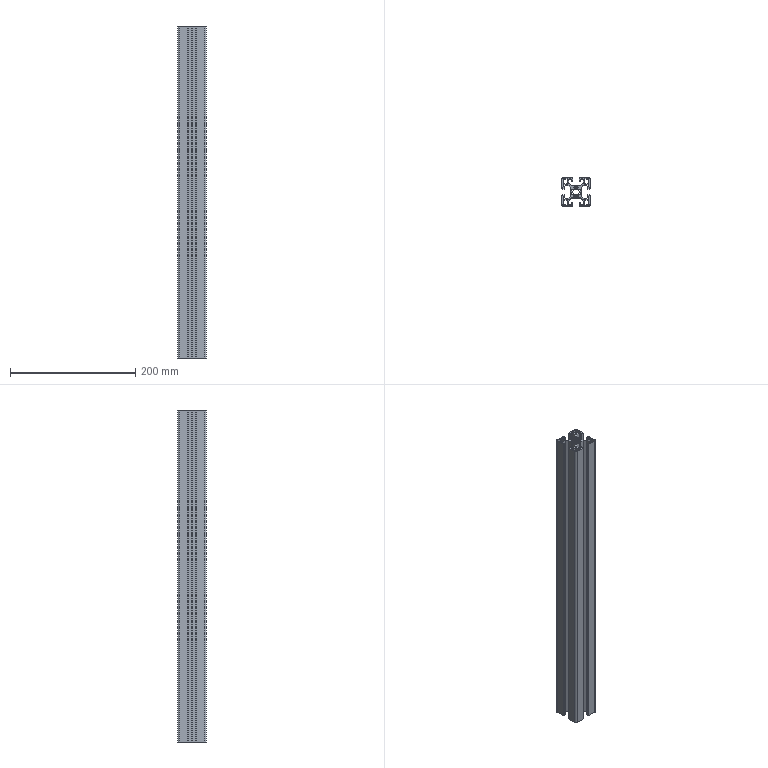Part | STEP file | PN_0041 | 1 solid | 271 faces | box 45 x 45 x 530 mm | volume 340057 mm3 | cylinder 149 | plane 122 | commonest cylinder face diameters 0.6 x48 1 x40 2 x28 10.2 x9 0.4 x8 16 x8